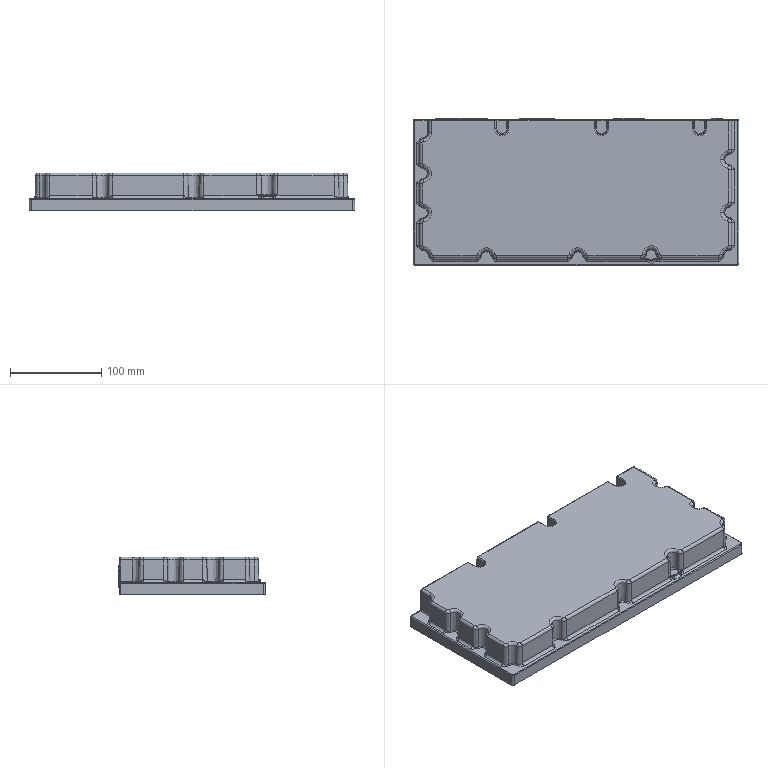Part | SolidWorks | features BaseBody 1 | 1 solid | 4611 faces | volume 826456 mm3 | torus 1469 | cylinder 996 | plane 756 | cone 734 | spline 590 | sphere 66 | commonest cylinder face diameters 1.005 x292 4.022 x144 1.006 x131 2.011 x107 1 x86 0.603 x55